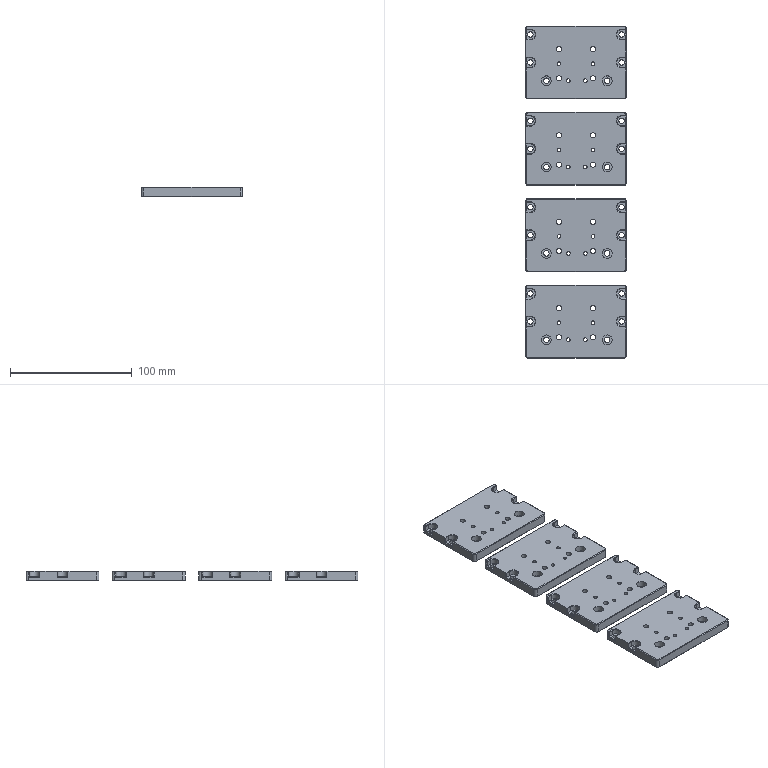CAM job | NX | 3-axis milling, drilling | part box 83 x 273 x 8 mm | stock box 89 x 279 x 8 mm
Tools:
number,name,description,diameter,corner_radius,flute_length,length,flutes
20,D10,Milling Tool-5 Parameters,10.0,0.0,50.0,75.0,2
22,D6A45,Milling Tool-5 Parameters,6.0,0.0,3.0,3.0,2
24,4.5ZT,Drilling Tool,4.5,0.0,35.0,50.0,2
17,D6,Milling Tool-5 Parameters,6.0,0.0,50.0,75.0,2
11,D10JING,Milling Tool-5 Parameters,10.0,0.0,50.0,75.0,2
21,4.2ZT,Drilling Tool,4.2,0.0,35.0,50.0,2
12,D2,Milling Tool-5 Parameters,2.0,0.0,50.0,75.0,2
Operations:
program,operation,operation_type,tool,method,geometry_group,spindle_rpm,surface_speed,feed_per_tooth,feed_cut,feed_plunge,cut_length_mm,path_length_mm,cut_time_min,machine_time_min
1AB胶-90-280-8毛胚,DRILLING_COPY_1_COPY_1,Operation,D6A45,METHOD,A,5000.0,94.0,0.025,250.0,0.0,224.0,1637.494,0.896,1.037
1AB胶-90-280-8毛胚,DRILLING_COPY_1_COPY_COPY_COPY_COPY_1_COPY_COPY_1,Operation,4.2ZT,METHOD,A,2000.0,20.0,0.0375,150.0,0.0,220.189,1000.747,1.468,1.546
1AB胶-90-280-8毛胚,DRILLING_COPY_1_COPY_COPY_COPY_COPY_1_COPY_COPY_1_COPY,Operation,4.5ZT,METHOD,A,2000.0,20.0,0.0375,150.0,0.0,320.447,1376.154,2.136,2.242
1AB胶-90-280-8毛胚,ZLEVEL_PROFILE_COPY,ZLevelMilling,D10,METHOD,A,7500.0,235.0,0.1667,2500.0,100.0,10471.08,11158.193,4.188,4.257
1AB胶-90-280-8毛胚,HOLE_MILLING_COPY,CylinderMilling,D6,METHOD,A,7500.0,141.0,0.0933,1400.0,100.0,717.581,1643.38,0.5126,0.6051
1AB胶-90-280-8毛胚,FLOOR_WALL,VolumeBased25DMillingOperation,D6,METHOD,A,9500.0,179.0,0.0947,1800.0,100.0,3453.333,5721.703,1.919,2.145
1AB胶-90-280-8毛胚,ZLEVEL_PROFILE_COPY_COPY,ZLevelMilling,D2,METHOD,A,7500.0,47.0,0.0667,1000.0,100.0,2386.34,3845.485,2.386,2.532
1AB胶-90-280-8毛胚,ZLEVEL_PROFILE_1_COPY_1_COPY_COPY,ZLevelMilling,D6A45,METHOD,A,7500.0,141.0,0.0667,1000.0,100.0,1848.671,6764.987,1.849,2.34
1AB胶-90-280-8毛胚,刀补12,ZLevelMilling,D2,METHOD,A,7500.0,47.0,0.0667,1000.0,100.0,378.912,1845.433,0.3789,0.5256
1AB胶-90-280-8毛胚,ZLEVEL_PROFILE_COPY_COPY_1,ZLevelMilling,D10JING,METHOD,A,7500.0,235.0,0.0667,1000.0,100.0,3929.186,4554.665,3.929,3.992